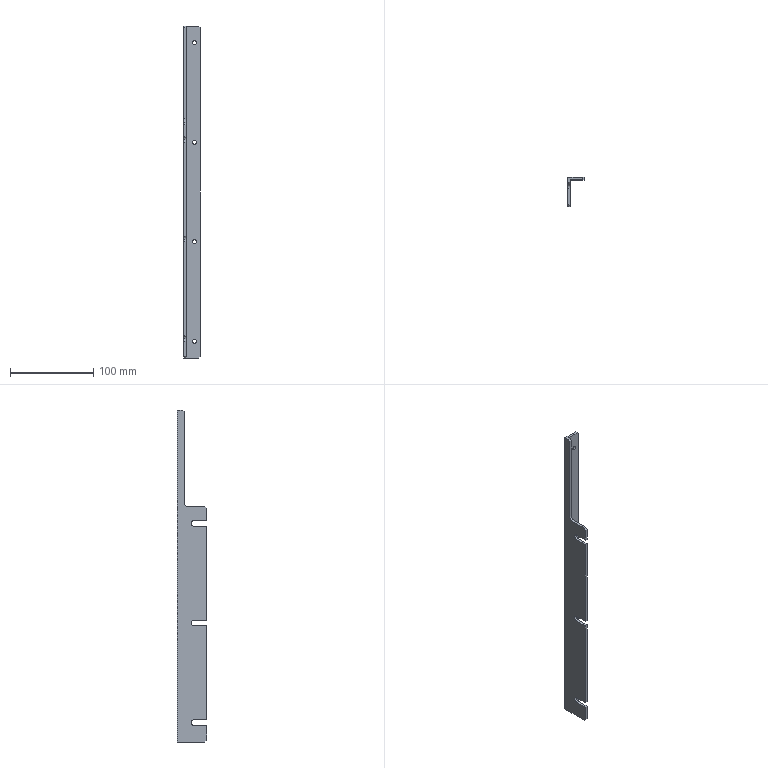Part | SolidWorks | features BaseBody 1 | 1 solid | 39 faces | box 20 x 35 x 400 mm | volume 51653 mm3 | plane 24 | cylinder 15 | commonest cylinder face diameters 5 x8 6.6 x6 10 x1
STEP:
#1=CARTESIAN_POINT('',(13.,32.,377.5));
#2=VERTEX_POINT('',#1);
#3=CARTESIAN_POINT('',(13.,32.,382.5));
#4=VERTEX_POINT('',#3);
#5=CARTESIAN_POINT('',(13.,32.,380.));
#6=DIRECTION('',(0.,1.,0.));
#7=DIRECTION('',(0.,0.,1.));
#8=AXIS2_PLACEMENT_3D('',#5,#6,#7);
#9=CIRCLE('',#8,2.5);
#10=EDGE_CURVE('',#2,#4,#9,.T.);
#11=ORIENTED_EDGE('',*,*,#10,.F.);
#12=CARTESIAN_POINT('',(13.,35.,377.5));
#13=VERTEX_POINT('',#12);
#14=CARTESIAN_POINT('',(13.,35.,377.5));
#15=DIRECTION('',(0.,1.,0.));
#16=VECTOR('',#15,1000.);
#17=LINE('',#14,#16);
#18=EDGE_CURVE('',#2,#13,#17,.T.);
#19=ORIENTED_EDGE('',*,*,#18,.T.);
#20=CARTESIAN_POINT('',(13.,35.,382.5));
#21=VERTEX_POINT('',#20);
#22=CARTESIAN_POINT('',(13.,35.,380.));
#23=DIRECTION('',(0.,1.,0.));
#24=DIRECTION('',(0.,0.,1.));
#25=AXIS2_PLACEMENT_3D('',#22,#23,#24);
#26=CIRCLE('',#25,2.5);
#27=EDGE_CURVE('',#13,#21,#26,.T.);
#28=ORIENTED_EDGE('',*,*,#27,.T.);
#29=CARTESIAN_POINT('',(13.,35.,382.5));
#30=DIRECTION('',(0.,1.,0.));
#31=VECTOR('',#30,1000.);
#32=LINE('',#29,#31);
#33=EDGE_CURVE('',#4,#21,#32,.T.);
#34=ORIENTED_EDGE('',*,*,#33,.F.);
#35=EDGE_LOOP('',(#11,#19,#28,#34));
#36=FACE_OUTER_BOUND('',#35,.T.);
#37=CARTESIAN_POINT('',(13.,35.,380.));
#38=DIRECTION('',(0.,1.,0.));
#39=DIRECTION('',(0.,0.,1.));
#40=AXIS2_PLACEMENT_3D('',#37,#38,#39);
#41=CYLINDRICAL_SURFACE('',#40,2.5);
#42=ADVANCED_FACE('',(#36),#41,.F.);
#43=CARTESIAN_POINT('',(13.,32.,257.5));
#44=VERTEX_POINT('',#43);
#45=CARTESIAN_POINT('',(13.,32.,262.5));
#46=VERTEX_POINT('',#45);
#47=CARTESIAN_POINT('',(13.,32.,260.));
#48=DIRECTION('',(0.,1.,0.));
#49=DIRECTION('',(0.,0.,1.));
#50=AXIS2_PLACEMENT_3D('',#47,#48,#49);
#51=CIRCLE('',#50,2.5);
#52=EDGE_CURVE('',#44,#46,#51,.T.);
#53=ORIENTED_EDGE('',*,*,#52,.F.);
#54=CARTESIAN_POINT('',(13.,35.,257.5));
#55=VERTEX_POINT('',#54);
#56=CARTESIAN_POINT('',(13.,35.,257.5));
#57=DIRECTION('',(0.,1.,0.));
#58=VECTOR('',#57,1000.);
#59=LINE('',#56,#58);
#60=EDGE_CURVE('',#44,#55,#59,.T.);
#61=ORIENTED_EDGE('',*,*,#60,.T.);
#62=CARTESIAN_POINT('',(13.,35.,262.5));
#63=VERTEX_POINT('',#62);
#64=CARTESIAN_POINT('',(13.,35.,260.));
#65=DIRECTION('',(0.,1.,0.));
#66=DIRECTION('',(0.,0.,1.));
#67=AXIS2_PLACEMENT_3D('',#64,#65,#66);
#68=CIRCLE('',#67,2.5);
#69=EDGE_CURVE('',#55,#63,#68,.T.);
#70=ORIENTED_EDGE('',*,*,#69,.T.);
#71=CARTESIAN_POINT('',(13.,35.,262.5));
#72=DIRECTION('',(0.,1.,0.));
#73=VECTOR('',#72,1000.);
#74=LINE('',#71,#73);
#75=EDGE_CURVE('',#46,#63,#74,.T.);
#76=ORIENTED_EDGE('',*,*,#75,.F.);
#77=EDGE_LOOP('',(#53,#61,#70,#76));
#78=FACE_OUTER_BOUND('',#77,.T.);
#79=CARTESIAN_POINT('',(13.,35.,260.));
#80=DIRECTION('',(0.,1.,0.));
#81=DIRECTION('',(0.,0.,1.));
#82=AXIS2_PLACEMENT_3D('',#79,#80,#81);
#83=CYLINDRICAL_SURFACE('',#82,2.5);
#84=ADVANCED_FACE('',(#78),#83,.F.);
#85=CARTESIAN_POINT('',(13.,32.,137.5));
#86=VERTEX_POINT('',#85);
#87=CARTESIAN_POINT('',(13.,32.,142.5));
#88=VERTEX_POINT('',#87);
#89=CARTESIAN_POINT('',(13.,32.,140.));
#90=DIRECTION('',(0.,1.,0.));
#91=DIRECTION('',(0.,0.,1.));
#92=AXIS2_PLACEMENT_3D('',#89,#90,#91);
#93=CIRCLE('',#92,2.5);
#94=EDGE_CURVE('',#86,#88,#93,.T.);
#95=ORIENTED_EDGE('',*,*,#94,.F.);
#96=CARTESIAN_POINT('',(13.,35.,137.5));
#97=VERTEX_POINT('',#96);
#98=CARTESIAN_POINT('',(13.,35.,137.5));
#99=DIRECTION('',(0.,1.,0.));
#100=VECTOR('',#99,1000.);
#101=LINE('',#98,#100);
#102=EDGE_CURVE('',#86,#97,#101,.T.);
#103=ORIENTED_EDGE('',*,*,#102,.T.);
#104=CARTESIAN_POINT('',(13.,35.,142.5));
#105=VERTEX_POINT('',#104);
#106=CARTESIAN_POINT('',(13.,35.,140.));
#107=DIRECTION('',(0.,1.,0.));
#108=DIRECTION('',(0.,0.,1.));
#109=AXIS2_PLACEMENT_3D('',#106,#107,#108);
#110=CIRCLE('',#109,2.5);
#111=EDGE_CURVE('',#97,#105,#110,.T.);
#112=ORIENTED_EDGE('',*,*,#111,.T.);
#113=CARTESIAN_POINT('',(13.,35.,142.5));
#114=DIRECTION('',(0.,1.,0.));
#115=VECTOR('',#114,1000.);
#116=LINE('',#113,#115);
#117=EDGE_CURVE('',#88,#105,#116,.T.);
#118=ORIENTED_EDGE('',*,*,#117,.F.);
#119=EDGE_LOOP('',(#95,#103,#112,#118));
#120=FACE_OUTER_BOUND('',#119,.T.);
#121=CARTESIAN_POINT('',(13.,35.,140.));
#122=DIRECTION('',(0.,1.,0.));
#123=DIRECTION('',(0.,0.,1.));
#124=AXIS2_PLACEMENT_3D('',#121,#122,#123);
#125=CYLINDRICAL_SURFACE('',#124,2.5);
#126=ADVANCED_FACE('',(#120),#125,.F.);
#127=CARTESIAN_POINT('',(13.,32.,17.5));
#128=VERTEX_POINT('',#127);
#129=CARTESIAN_POINT('',(13.,32.,22.5));
#130=VERTEX_POINT('',#129);
#131=CARTESIAN_POINT('',(13.,32.,20.));
#132=DIRECTION('',(0.,1.,0.));
#133=DIRECTION('',(0.,0.,1.));
#134=AXIS2_PLACEMENT_3D('',#131,#132,#133);
#135=CIRCLE('',#134,2.5);
#136=EDGE_CURVE('',#128,#130,#135,.T.);
#137=ORIENTED_EDGE('',*,*,#136,.F.);
#138=CARTESIAN_POINT('',(13.,35.,17.5));
#139=VERTEX_POINT('',#138);
#140=CARTESIAN_POINT('',(13.,35.,17.5));
#141=DIRECTION('',(0.,1.,0.));
#142=VECTOR('',#141,1000.);
#143=LINE('',#140,#142);
#144=EDGE_CURVE('',#128,#139,#143,.T.);
#145=ORIENTED_EDGE('',*,*,#144,.T.);
#146=CARTESIAN_POINT('',(13.,35.,22.5));
#147=VERTEX_POINT('',#146);
#148=CARTESIAN_POINT('',(13.,35.,20.));
#149=DIRECTION('',(0.,1.,0.));
#150=DIRECTION('',(0.,0.,1.));
#151=AXIS2_PLACEMENT_3D('',#148,#149,#150);
#152=CIRCLE('',#151,2.5);
#153=EDGE_CURVE('',#139,#147,#152,.T.);
#154=ORIENTED_EDGE('',*,*,#153,.T.);
#155=CARTESIAN_POINT('',(13.,35.,22.5));
#156=DIRECTION('',(0.,1.,0.));
#157=VECTOR('',#156,1000.);
#158=LINE('',#155,#157);
#159=EDGE_CURVE('',#130,#147,#158,.T.);
#160=ORIENTED_EDGE('',*,*,#159,.F.);
#161=EDGE_LOOP('',(#137,#145,#154,#160));
#162=FACE_OUTER_BOUND('',#161,.T.);
#163=CARTESIAN_POINT('',(13.,35.,20.));
#164=DIRECTION('',(0.,1.,0.));
#165=DIRECTION('',(0.,0.,1.));
#166=AXIS2_PLACEMENT_3D('',#163,#164,#165);
#167=CYLINDRICAL_SURFACE('',#166,2.5);
#168=ADVANCED_FACE('',(#162),#167,.F.);
#169=CARTESIAN_POINT('',(0.,18.3,23.3));
#170=VERTEX_POINT('',#169);
#171=CARTESIAN_POINT('',(0.,15.,26.6));
#172=VERTEX_POINT('',#171);
#173=CARTESIAN_POINT('',(0.,15.,23.3));
#174=DIRECTION('',(1.,0.,0.));
#175=DIRECTION('',(0.,1.,0.));
#176=AXIS2_PLACEMENT_3D('',#173,#174,#175);
#177=CIRCLE('',#176,3.3);
#178=EDGE_CURVE('',#170,#172,#177,.T.);
#179=ORIENTED_EDGE('',*,*,#178,.F.);
#180=CARTESIAN_POINT('',(3.,18.3,23.3));
#181=VERTEX_POINT('',#180);
#182=CARTESIAN_POINT('',(0.,18.3,23.3));
#183=DIRECTION('',(1.,0.,0.));
#184=VECTOR('',#183,1000.);
#185=LINE('',#182,#184);
#186=EDGE_CURVE('',#170,#181,#185,.T.);
#187=ORIENTED_EDGE('',*,*,#186,.T.);
#188=CARTESIAN_POINT('',(3.,15.,26.6));
#189=VERTEX_POINT('',#188);
#190=CARTESIAN_POINT('',(3.,15.,23.3));
#191=DIRECTION('',(1.,0.,0.));
#192=DIRECTION('',(0.,1.,0.));
#193=AXIS2_PLACEMENT_3D('',#190,#191,#192);
#194=CIRCLE('',#193,3.3);
#195=EDGE_CURVE('',#181,#189,#194,.T.);
#196=ORIENTED_EDGE('',*,*,#195,.T.);
#197=CARTESIAN_POINT('',(0.,15.,26.6));
#198=DIRECTION('',(1.,0.,0.));
#199=VECTOR('',#198,1000.);
#200=LINE('',#197,#199);
#201=EDGE_CURVE('',#172,#189,#200,.T.);
#202=ORIENTED_EDGE('',*,*,#201,.F.);
#203=EDGE_LOOP('',(#179,#187,#196,#202));
#204=FACE_OUTER_BOUND('',#203,.T.);
#205=CARTESIAN_POINT('',(0.,15.,23.3));
#206=DIRECTION('',(1.,0.,0.));
#207=DIRECTION('',(0.,1.,0.));
#208=AXIS2_PLACEMENT_3D('',#205,#206,#207);
#209=CYLINDRICAL_SURFACE('',#208,3.3);
#210=ADVANCED_FACE('',(#204),#209,.F.);
#211=CARTESIAN_POINT('',(0.,18.3,263.3));
#212=VERTEX_POINT('',#211);
#213=CARTESIAN_POINT('',(0.,15.,266.6));
#214=VERTEX_POINT('',#213);
#215=CARTESIAN_POINT('',(0.,15.,263.3));
#216=DIRECTION('',(1.,0.,0.));
#217=DIRECTION('',(0.,1.,0.));
#218=AXIS2_PLACEMENT_3D('',#215,#216,#217);
#219=CIRCLE('',#218,3.3);
#220=EDGE_CURVE('',#212,#214,#219,.T.);
#221=ORIENTED_EDGE('',*,*,#220,.F.);
#222=CARTESIAN_POINT('',(3.,18.3,263.3));
#223=VERTEX_POINT('',#222);
#224=CARTESIAN_POINT('',(0.,18.3,263.3));
#225=DIRECTION('',(1.,0.,0.));
#226=VECTOR('',#225,1000.);
#227=LINE('',#224,#226);
#228=EDGE_CURVE('',#212,#223,#227,.T.);
#229=ORIENTED_EDGE('',*,*,#228,.T.);
#230=CARTESIAN_POINT('',(3.,15.,266.6));
#231=VERTEX_POINT('',#230);
#232=CARTESIAN_POINT('',(3.,15.,263.3));
#233=DIRECTION('',(1.,0.,0.));
#234=DIRECTION('',(0.,1.,0.));
#235=AXIS2_PLACEMENT_3D('',#232,#233,#234);
#236=CIRCLE('',#235,3.3);
#237=EDGE_CURVE('',#223,#231,#236,.T.);
#238=ORIENTED_EDGE('',*,*,#237,.T.);
#239=CARTESIAN_POINT('',(0.,15.,266.6));
#240=DIRECTION('',(1.,0.,0.));
#241=VECTOR('',#240,1000.);
#242=LINE('',#239,#241);
#243=EDGE_CURVE('',#214,#231,#242,.T.);
#244=ORIENTED_EDGE('',*,*,#243,.F.);
#245=EDGE_LOOP('',(#221,#229,#238,#244));
#246=FACE_OUTER_BOUND('',#245,.T.);
#247=CARTESIAN_POINT('',(0.,15.,263.3));
#248=DIRECTION('',(1.,0.,0.));
#249=DIRECTION('',(0.,1.,0.));
#250=AXIS2_PLACEMENT_3D('',#247,#248,#249);
#251=CYLINDRICAL_SURFACE('',#250,3.3);
#252=ADVANCED_FACE('',(#246),#251,.F.);
#253=CARTESIAN_POINT('',(0.,18.3,143.3));
#254=VERTEX_POINT('',#253);
#255=CARTESIAN_POINT('',(0.,15.,146.6));
#256=VERTEX_POINT('',#255);
#257=CARTESIAN_POINT('',(0.,15.,143.3));
#258=DIRECTION('',(1.,0.,0.));
#259=DIRECTION('',(0.,1.,0.));
#260=AXIS2_PLACEMENT_3D('',#257,#258,#259);
#261=CIRCLE('',#260,3.3);
#262=EDGE_CURVE('',#254,#256,#261,.T.);
#263=ORIENTED_EDGE('',*,*,#262,.F.);
#264=CARTESIAN_POINT('',(3.,18.3,143.3));
#265=VERTEX_POINT('',#264);
#266=CARTESIAN_POINT('',(0.,18.3,143.3));
#267=DIRECTION('',(1.,0.,0.));
#268=VECTOR('',#267,1000.);
#269=LINE('',#266,#268);
#270=EDGE_CURVE('',#254,#265,#269,.T.);
#271=ORIENTED_EDGE('',*,*,#270,.T.);
#272=CARTESIAN_POINT('',(3.,15.,146.6));
#273=VERTEX_POINT('',#272);
#274=CARTESIAN_POINT('',(3.,15.,143.3));
#275=DIRECTION('',(1.,0.,0.));
#276=DIRECTION('',(0.,1.,0.));
#277=AXIS2_PLACEMENT_3D('',#274,#275,#276);
#278=CIRCLE('',#277,3.3);
#279=EDGE_CURVE('',#265,#273,#278,.T.);
#280=ORIENTED_EDGE('',*,*,#279,.T.);
#281=CARTESIAN_POINT('',(0.,15.,146.6));
#282=DIRECTION('',(1.,0.,0.));
#283=VECTOR('',#282,1000.);
#284=LINE('',#281,#283);
#285=EDGE_CURVE('',#256,#273,#284,.T.);
#286=ORIENTED_EDGE('',*,*,#285,.F.);
#287=EDGE_LOOP('',(#263,#271,#280,#286));
#288=FACE_OUTER_BOUND('',#287,.T.);
#289=CARTESIAN_POINT('',(0.,15.,143.3));
#290=DIRECTION('',(1.,0.,0.));
#291=DIRECTION('',(0.,1.,0.));
#292=AXIS2_PLACEMENT_3D('',#289,#290,#291);
#293=CYLINDRICAL_SURFACE('',#292,3.3);
#294=ADVANCED_FACE('',(#288),#293,.F.);
#295=CARTESIAN_POINT('',(0.,22.,283.3));
#296=VERTEX_POINT('',#295);
#297=CARTESIAN_POINT('',(0.,27.,288.3));
#298=VERTEX_POINT('',#297);
#299=CARTESIAN_POINT('',(0.,22.,288.3));
#300=DIRECTION('',(1.,0.,0.));
#301=DIRECTION('',(0.,0.,-1.));
#302=AXIS2_PLACEMENT_3D('',#299,#300,#301);
#303=CIRCLE('',#302,5.);
#304=EDGE_CURVE('',#296,#298,#303,.T.);
#305=ORIENTED_EDGE('',*,*,#304,.F.);
#306=CARTESIAN_POINT('',(3.,22.,283.3));
#307=VERTEX_POINT('',#306);
#308=CARTESIAN_POINT('',(0.,22.,283.3));
#309=DIRECTION('',(-1.,0.,0.));
#310=VECTOR('',#309,1000.);
#311=LINE('',#308,#310);
#312=EDGE_CURVE('',#307,#296,#311,.T.);
#313=ORIENTED_EDGE('',*,*,#312,.F.);
#314=CARTESIAN_POINT('',(3.,27.,288.3));
#315=VERTEX_POINT('',#314);
#316=CARTESIAN_POINT('',(3.,22.,288.3));
#317=DIRECTION('',(-1.,0.,0.));
#318=DIRECTION('',(0.,-1.,0.));
#319=AXIS2_PLACEMENT_3D('',#316,#317,#318);
#320=CIRCLE('',#319,5.);
#321=EDGE_CURVE('',#315,#307,#320,.T.);
#322=ORIENTED_EDGE('',*,*,#321,.F.);
#323=CARTESIAN_POINT('',(3.,27.,288.3));
#324=DIRECTION('',(1.,0.,0.));
#325=VECTOR('',#324,1000.);
#326=LINE('',#323,#325);
#327=EDGE_CURVE('',#298,#315,#326,.T.);
#328=ORIENTED_EDGE('',*,*,#327,.F.);
#329=EDGE_LOOP('',(#305,#313,#322,#328));
#330=FACE_OUTER_BOUND('',#329,.T.);
#331=CARTESIAN_POINT('',(0.,22.,288.3));
#332=DIRECTION('',(-1.,0.,0.));
#333=DIRECTION('',(0.,-1.,0.));
#334=AXIS2_PLACEMENT_3D('',#331,#332,#333);
#335=CYLINDRICAL_SURFACE('',#334,5.);
#336=ADVANCED_FACE('',(#330),#335,.F.);
#337=CARTESIAN_POINT('',(18.,32.,0.));
#338=VERTEX_POINT('',#337);
#339=CARTESIAN_POINT('',(20.,32.,2.));
#340=VERTEX_POINT('',#339);
#341=CARTESIAN_POINT('',(20.,32.,2.));
#342=DIRECTION('',(0.7071,0.,0.7071));
#343=VECTOR('',#342,1000.);
#344=LINE('',#341,#343);
#345=EDGE_CURVE('',#338,#340,#344,.T.);
#346=ORIENTED_EDGE('',*,*,#345,.F.);
#347=CARTESIAN_POINT('',(18.,35.,0.));
#348=VERTEX_POINT('',#347);
#349=CARTESIAN_POINT('',(18.,32.,0.));
#350=DIRECTION('',(0.,-1.,0.));
#351=VECTOR('',#350,1000.);
#352=LINE('',#349,#351);
#353=EDGE_CURVE('',#348,#338,#352,.T.);
#354=ORIENTED_EDGE('',*,*,#353,.F.);
#355=CARTESIAN_POINT('',(20.,35.,2.));
#356=VERTEX_POINT('',#355);
#357=CARTESIAN_POINT('',(20.,35.,2.));
#358=DIRECTION('',(-0.7071,0.,-0.7071));
#359=VECTOR('',#358,1000.);
#360=LINE('',#357,#359);
#361=EDGE_CURVE('',#356,#348,#360,.T.);
#362=ORIENTED_EDGE('',*,*,#361,.F.);
#363=CARTESIAN_POINT('',(20.,35.,2.));
#364=DIRECTION('',(0.,1.,0.));
#365=VECTOR('',#364,1000.);
#366=LINE('',#363,#365);
#367=EDGE_CURVE('',#340,#356,#366,.T.);
#368=ORIENTED_EDGE('',*,*,#367,.F.);
#369=EDGE_LOOP('',(#346,#354,#362,#368));
#370=FACE_OUTER_BOUND('',#369,.T.);
#371=CARTESIAN_POINT('',(20.,35.,2.));
#372=DIRECTION('',(0.7071,0.,-0.7071));
#373=DIRECTION('',(0.,-1.,0.));
#374=AXIS2_PLACEMENT_3D('',#371,#372,#373);
#375=PLANE('',#374);
#376=ADVANCED_FACE('',(#370),#375,.T.);
#377=CARTESIAN_POINT('',(20.,32.,398.));
#378=VERTEX_POINT('',#377);
#379=CARTESIAN_POINT('',(18.,32.,400.));
#380=VERTEX_POINT('',#379);
#381=CARTESIAN_POINT('',(18.,32.,400.));
#382=DIRECTION('',(-0.7071,0.,0.7071));
#383=VECTOR('',#382,1000.);
#384=LINE('',#381,#383);
#385=EDGE_CURVE('',#378,#380,#384,.T.);
#386=ORIENTED_EDGE('',*,*,#385,.F.);
#387=CARTESIAN_POINT('',(20.,35.,398.));
#388=VERTEX_POINT('',#387);
#389=CARTESIAN_POINT('',(20.,35.,398.));
#390=DIRECTION('',(0.,-1.,0.));
#391=VECTOR('',#390,1000.);
#392=LINE('',#389,#391);
#393=EDGE_CURVE('',#388,#378,#392,.T.);
#394=ORIENTED_EDGE('',*,*,#393,.F.);
#395=CARTESIAN_POINT('',(18.,35.,400.));
#396=VERTEX_POINT('',#395);
#397=CARTESIAN_POINT('',(18.,35.,400.));
#398=DIRECTION('',(0.7071,0.,-0.7071));
#399=VECTOR('',#398,1000.);
#400=LINE('',#397,#399);
#401=EDGE_CURVE('',#396,#388,#400,.T.);
#402=ORIENTED_EDGE('',*,*,#401,.F.);
#403=CARTESIAN_POINT('',(18.,0.,400.));
#404=DIRECTION('',(0.,1.,0.));
#405=VECTOR('',#404,1000.);
#406=LINE('',#403,#405);
#407=EDGE_CURVE('',#380,#396,#406,.T.);
#408=ORIENTED_EDGE('',*,*,#407,.F.);
#409=EDGE_LOOP('',(#386,#394,#402,#408));
#410=FACE_OUTER_BOUND('',#409,.T.);
#411=CARTESIAN_POINT('',(18.,0.,400.));
#412=DIRECTION('',(-0.7071,0.,-0.7071));
#413=DIRECTION('',(-0.7071,0.,0.7071));
#414=AXIS2_PLACEMENT_3D('',#411,#412,#413);
#415=PLANE('',#414);
#416=ADVANCED_FACE('',(#410),#415,.F.);
#417=CARTESIAN_POINT('',(0.,27.,398.));
#418=VERTEX_POINT('',#417);
#419=CARTESIAN_POINT('',(0.,29.,400.));
#420=VERTEX_POINT('',#419);
#421=CARTESIAN_POINT('',(0.,29.,400.));
#422=DIRECTION('',(0.,0.7071,0.7071));
#423=VECTOR('',#422,1000.);
#424=LINE('',#421,#423);
#425=EDGE_CURVE('',#418,#420,#424,.T.);
#426=ORIENTED_EDGE('',*,*,#425,.F.);
#427=CARTESIAN_POINT('',(3.,27.,398.));
#428=VERTEX_POINT('',#427);
#429=CARTESIAN_POINT('',(0.,27.,398.));
#430=DIRECTION('',(-1.,0.,0.));
#431=VECTOR('',#430,1000.);
#432=LINE('',#429,#431);
#433=EDGE_CURVE('',#428,#418,#432,.T.);
#434=ORIENTED_EDGE('',*,*,#433,.F.);
#435=CARTESIAN_POINT('',(3.,29.,400.));
#436=VERTEX_POINT('',#435);
#437=CARTESIAN_POINT('',(3.,29.,400.));
#438=DIRECTION('',(0.,-0.7071,-0.7071));
#439=VECTOR('',#438,1000.);
#440=LINE('',#437,#439);
#441=EDGE_CURVE('',#436,#428,#440,.T.);
#442=ORIENTED_EDGE('',*,*,#441,.F.);
#443=CARTESIAN_POINT('',(0.,29.,400.));
#444=DIRECTION('',(1.,0.,0.));
#445=VECTOR('',#444,1000.);
#446=LINE('',#443,#445);
#447=EDGE_CURVE('',#420,#436,#446,.T.);
#448=ORIENTED_EDGE('',*,*,#447,.F.);
#449=EDGE_LOOP('',(#426,#434,#442,#448));
#450=FACE_OUTER_BOUND('',#449,.T.);
#451=CARTESIAN_POINT('',(0.,29.,400.));
#452=DIRECTION('',(0.,0.7071,-0.7071));
#453=DIRECTION('',(-1.,0.,0.));
#454=AXIS2_PLACEMENT_3D('',#451,#452,#453);
#455=PLANE('',#454);
#456=ADVANCED_FACE('',(#450),#455,.F.);
#457=CARTESIAN_POINT('',(0.,0.,281.3));
#458=VERTEX_POINT('',#457);
#459=CARTESIAN_POINT('',(0.,2.,283.3));
#460=VERTEX_POINT('',#459);
#461=CARTESIAN_POINT('',(0.,2.,283.3));
#462=DIRECTION('',(0.,0.7071,0.7071));
#463=VECTOR('',#462,1000.);
#464=LINE('',#461,#463);
#465=EDGE_CURVE('',#458,#460,#464,.T.);
#466=ORIENTED_EDGE('',*,*,#465,.F.);
#467=CARTESIAN_POINT('',(3.,0.,281.3));
#468=VERTEX_POINT('',#467);
#469=CARTESIAN_POINT('',(3.,0.,281.3));
#470=DIRECTION('',(-1.,0.,0.));
#471=VECTOR('',#470,1000.);
#472=LINE('',#469,#471);
#473=EDGE_CURVE('',#468,#458,#472,.T.);
#474=ORIENTED_EDGE('',*,*,#473,.F.);
#475=CARTESIAN_POINT('',(3.,2.,283.3));
#476=VERTEX_POINT('',#475);
#477=CARTESIAN_POINT('',(3.,2.,283.3));
#478=DIRECTION('',(0.,-0.7071,-0.7071));
#479=VECTOR('',#478,1000.);
#480=LINE('',#477,#479);
#481=EDGE_CURVE('',#476,#468,#480,.T.);
#482=ORIENTED_EDGE('',*,*,#481,.F.);
#483=CARTESIAN_POINT('',(0.,2.,283.3));
#484=DIRECTION('',(1.,0.,0.));
#485=VECTOR('',#484,1000.);
#486=LINE('',#483,#485);
#487=EDGE_CURVE('',#460,#476,#486,.T.);
#488=ORIENTED_EDGE('',*,*,#487,.F.);
#489=EDGE_LOOP('',(#466,#474,#482,#488));
#490=FACE_OUTER_BOUND('',#489,.T.);
#491=CARTESIAN_POINT('',(0.,2.,283.3));
#492=DIRECTION('',(0.,0.7071,-0.7071));
#493=DIRECTION('',(-1.,0.,0.));
#494=AXIS2_PLACEMENT_3D('',#491,#492,#493);
#495=PLANE('',#494);
#496=ADVANCED_FACE('',(#490),#495,.F.);
#497=CARTESIAN_POINT('',(0.,2.,0.));
#498=VERTEX_POINT('',#497);
#499=CARTESIAN_POINT('',(0.,0.,2.));
#500=VERTEX_POINT('',#499);
#501=CARTESIAN_POINT('',(0.,0.,2.));
#502=DIRECTION('',(0.,-0.7071,0.7071));
#503=VECTOR('',#502,1000.);
#504=LINE('',#501,#503);
#505=EDGE_CURVE('',#498,#500,#504,.T.);
#506=ORIENTED_EDGE('',*,*,#505,.F.);
#507=CARTESIAN_POINT('',(3.,2.,0.));
#508=VERTEX_POINT('',#507);
#509=CARTESIAN_POINT('',(0.,2.,0.));
#510=DIRECTION('',(-1.,0.,0.));
#511=VECTOR('',#510,1000.);
#512=LINE('',#509,#511);
#513=EDGE_CURVE('',#508,#498,#512,.T.);
#514=ORIENTED_EDGE('',*,*,#513,.F.);
#515=CARTESIAN_POINT('',(3.,0.,2.));
#516=VERTEX_POINT('',#515);
#517=CARTESIAN_POINT('',(3.,0.,2.));
#518=DIRECTION('',(0.,0.7071,-0.7071));
#519=VECTOR('',#518,1000.);
#520=LINE('',#517,#519);
#521=EDGE_CURVE('',#516,#508,#520,.T.);
#522=ORIENTED_EDGE('',*,*,#521,.F.);
#523=CARTESIAN_POINT('',(3.,0.,2.));
#524=DIRECTION('',(1.,0.,0.));
#525=VECTOR('',#524,1000.);
#526=LINE('',#523,#525);
#527=EDGE_CURVE('',#500,#516,#526,.T.);
#528=ORIENTED_EDGE('',*,*,#527,.F.);
#529=EDGE_LOOP('',(#506,#514,#522,#528));
#530=FACE_OUTER_BOUND('',#529,.T.);
#531=CARTESIAN_POINT('',(3.,0.,2.));
#532=DIRECTION('',(0.,-0.7071,-0.7071));
#533=DIRECTION('',(0.,-0.7071,0.7071));
#534=AXIS2_PLACEMENT_3D('',#531,#532,#533);
#535=PLANE('',#534);
#536=ADVANCED_FACE('',(#530),#535,.T.);
#537=CARTESIAN_POINT('',(0.,27.,283.3));
#538=DIRECTION('',(0.,0.,1.));
#539=VECTOR('',#538,1000.);
#540=LINE('',#537,#539);
#541=EDGE_CURVE('',#298,#418,#540,.T.);
#542=ORIENTED_EDGE('',*,*,#541,.F.);
#543=ORIENTED_EDGE('',*,*,#327,.T.);
#544=CARTESIAN_POINT('',(3.,27.,283.3));
#545=DIRECTION('',(0.,0.,1.));
#546=VECTOR('',#545,1000.);
#547=LINE('',#544,#546);
#548=EDGE_CURVE('',#315,#428,#547,.T.);
#549=ORIENTED_EDGE('',*,*,#548,.T.);
#550=ORIENTED_EDGE('',*,*,#433,.T.);
#551=EDGE_LOOP('',(#542,#543,#549,#550));
#552=FACE_OUTER_BOUND('',#551,.T.);
#553=CARTESIAN_POINT('',(0.,27.,283.3));
#554=DIRECTION('',(0.,1.,0.));
#555=DIRECTION('',(0.,0.,-1.));
#556=AXIS2_PLACEMENT_3D('',#553,#554,#555);
#557=PLANE('',#556);
#558=ADVANCED_FACE('',(#552),#557,.F.);
#559=CARTESIAN_POINT('',(3.,0.,283.3));
#560=DIRECTION('',(0.,1.,0.));
#561=VECTOR('',#560,1000.);
#562=LINE('',#559,#561);
#563=EDGE_CURVE('',#476,#307,#562,.T.);
#564=ORIENTED_EDGE('',*,*,#563,.T.);
#565=ORIENTED_EDGE('',*,*,#312,.T.);
#566=CARTESIAN_POINT('',(0.,0.,283.3));
#567=DIRECTION('',(0.,1.,0.));
#568=VECTOR('',#567,1000.);
#569=LINE('',#566,#568);
#570=EDGE_CURVE('',#460,#296,#569,.T.);
#571=ORIENTED_EDGE('',*,*,#570,.F.);
#572=ORIENTED_EDGE('',*,*,#487,.T.);
#573=EDGE_LOOP('',(#564,#565,#571,#572));
#574=FACE_OUTER_BOUND('',#573,.T.);
#575=CARTESIAN_POINT('',(0.,0.,283.3));
#576=DIRECTION('',(0.,0.,-1.));
#577=DIRECTION('',(0.,-1.,0.));
#578=AXIS2_PLACEMENT_3D('',#575,#576,#577);
#579=PLANE('',#578);
#580=ADVANCED_FACE('',(#574),#579,.F.);
#581=CARTESIAN_POINT('',(3.,0.,20.));
#582=VERTEX_POINT('',#581);
#583=CARTESIAN_POINT('',(3.,15.,20.));
#584=VERTEX_POINT('',#583);
#585=CARTESIAN_POINT('',(3.,0.,20.));
#586=DIRECTION('',(0.,1.,0.));
#587=VECTOR('',#586,1000.);
#588=LINE('',#585,#587);
#589=EDGE_CURVE('',#582,#584,#588,.T.);
#590=ORIENTED_EDGE('',*,*,#589,.T.);
#591=CARTESIAN_POINT('',(0.,15.,20.));
#592=VERTEX_POINT('',#591);
#593=CARTESIAN_POINT('',(0.,15.,20.));
#594=DIRECTION('',(1.,0.,0.));
#595=VECTOR('',#594,1000.);
#596=LINE('',#593,#595);
#597=EDGE_CURVE('',#592,#584,#596,.T.);
#598=ORIENTED_EDGE('',*,*,#597,.F.);
#599=CARTESIAN_POINT('',(0.,0.,20.));
#600=VERTEX_POINT('',#599);
#601=CARTESIAN_POINT('',(0.,0.,20.));
#602=DIRECTION('',(0.,1.,0.));
#603=VECTOR('',#602,1000.);
#604=LINE('',#601,#603);
#605=EDGE_CURVE('',#600,#592,#604,.T.);
#606=ORIENTED_EDGE('',*,*,#605,.F.);
#607=CARTESIAN_POINT('',(0.,0.,20.));
#608=DIRECTION('',(1.,0.,0.));
#609=VECTOR('',#608,1000.);
#610=LINE('',#607,#609);
#611=EDGE_CURVE('',#600,#582,#610,.T.);
#612=ORIENTED_EDGE('',*,*,#611,.T.);
#613=EDGE_LOOP('',(#590,#598,#606,#612));
#614=FACE_OUTER_BOUND('',#613,.T.);
#615=CARTESIAN_POINT('',(0.,0.,20.));
#616=DIRECTION('',(0.,0.,-1.));
#617=DIRECTION('',(0.,-1.,0.));
#618=AXIS2_PLACEMENT_3D('',#615,#616,#617);
#619=PLANE('',#618);
#620=ADVANCED_FACE('',(#614),#619,.F.);
#621=CARTESIAN_POINT('',(3.,0.,26.6));
#622=VERTEX_POINT('',#621);
#623=CARTESIAN_POINT('',(3.,0.,26.6));
#624=DIRECTION('',(0.,-1.,0.));
#625=VECTOR('',#624,1000.);
#626=LINE('',#623,#625);
#627=EDGE_CURVE('',#189,#622,#626,.T.);
#628=ORIENTED_EDGE('',*,*,#627,.T.);
#629=CARTESIAN_POINT('',(0.,0.,26.6));
#630=VERTEX_POINT('',#629);
#631=CARTESIAN_POINT('',(0.,0.,26.6));
#632=DIRECTION('',(1.,0.,0.));
#633=VECTOR('',#632,1000.);
#634=LINE('',#631,#633);
#635=EDGE_CURVE('',#630,#622,#634,.T.);
#636=ORIENTED_EDGE('',*,*,#635,.F.);
#637=CARTESIAN_POINT('',(0.,0.,26.6));
#638=DIRECTION('',(0.,-1.,0.));
#639=VECTOR('',#638,1000.);
#640=LINE('',#637,#639);
#641=EDGE_CURVE('',#172,#630,#640,.T.);
#642=ORIENTED_EDGE('',*,*,#641,.F.);
#643=ORIENTED_EDGE('',*,*,#201,.T.);
#644=EDGE_LOOP('',(#628,#636,#642,#643));
#645=FACE_OUTER_BOUND('',#644,.T.);
#646=CARTESIAN_POINT('',(0.,0.,26.6));
#647=DIRECTION('',(0.,0.,1.));
#648=DIRECTION('',(0.,-1.,0.));
#649=AXIS2_PLACEMENT_3D('',#646,#647,#648);
#650=PLANE('',#649);
#651=ADVANCED_FACE('',(#645),#650,.F.);
#652=CARTESIAN_POINT('',(3.,0.,260.));
#653=VERTEX_POINT('',#652);
#654=CARTESIAN_POINT('',(3.,15.,260.));
#655=VERTEX_POINT('',#654);
#656=CARTESIAN_POINT('',(3.,0.,260.));
#657=DIRECTION('',(0.,1.,0.));
#658=VECTOR('',#657,1000.);
#659=LINE('',#656,#658);
#660=EDGE_CURVE('',#653,#655,#659,.T.);
#661=ORIENTED_EDGE('',*,*,#660,.T.);
#662=CARTESIAN_POINT('',(0.,15.,260.));
#663=VERTEX_POINT('',#662);
#664=CARTESIAN_POINT('',(0.,15.,260.));
#665=DIRECTION('',(1.,0.,0.));
#666=VECTOR('',#665,1000.);
#667=LINE('',#664,#666);
#668=EDGE_CURVE('',#663,#655,#667,.T.);
#669=ORIENTED_EDGE('',*,*,#668,.F.);
#670=CARTESIAN_POINT('',(0.,0.,260.));
#671=VERTEX_POINT('',#670);
#672=CARTESIAN_POINT('',(0.,0.,260.));
#673=DIRECTION('',(0.,1.,0.));
#674=VECTOR('',#673,1000.);
#675=LINE('',#672,#674);
#676=EDGE_CURVE('',#671,#663,#675,.T.);
#677=ORIENTED_EDGE('',*,*,#676,.F.);
#678=CARTESIAN_POINT('',(0.,0.,260.));
#679=DIRECTION('',(1.,0.,0.));
#680=VECTOR('',#679,1000.);
#681=LINE('',#678,#680);
#682=EDGE_CURVE('',#671,#653,#681,.T.);
#683=ORIENTED_EDGE('',*,*,#682,.T.);
#684=EDGE_LOOP('',(#661,#669,#677,#683));
#685=FACE_OUTER_BOUND('',#684,.T.);
#686=CARTESIAN_POINT('',(0.,0.,260.));
#687=DIRECTION('',(0.,0.,-1.));
#688=DIRECTION('',(0.,-1.,0.));
#689=AXIS2_PLACEMENT_3D('',#686,#687,#688);
#690=PLANE('',#689);
#691=ADVANCED_FACE('',(#685),#690,.F.);
#692=CARTESIAN_POINT('',(3.,0.,266.6));
#693=VERTEX_POINT('',#692);
#694=CARTESIAN_POINT('',(3.,0.,266.6));
#695=DIRECTION('',(0.,-1.,0.));
#696=VECTOR('',#695,1000.);
#697=LINE('',#694,#696);
#698=EDGE_CURVE('',#231,#693,#697,.T.);
#699=ORIENTED_EDGE('',*,*,#698,.T.);
#700=CARTESIAN_POINT('',(0.,0.,266.6));
#701=VERTEX_POINT('',#700);
#702=CARTESIAN_POINT('',(0.,0.,266.6));
#703=DIRECTION('',(1.,0.,0.));
#704=VECTOR('',#703,1000.);
#705=LINE('',#702,#704);
#706=EDGE_CURVE('',#701,#693,#705,.T.);
#707=ORIENTED_EDGE('',*,*,#706,.F.);
#708=CARTESIAN_POINT('',(0.,0.,266.6));
#709=DIRECTION('',(0.,-1.,0.));
#710=VECTOR('',#709,1000.);
#711=LINE('',#708,#710);
#712=EDGE_CURVE('',#214,#701,#711,.T.);
#713=ORIENTED_EDGE('',*,*,#712,.F.);
#714=ORIENTED_EDGE('',*,*,#243,.T.);
#715=EDGE_LOOP('',(#699,#707,#713,#714));
#716=FACE_OUTER_BOUND('',#715,.T.);
#717=CARTESIAN_POINT('',(0.,0.,266.6));
#718=DIRECTION('',(0.,0.,1.));
#719=DIRECTION('',(1.,0.,0.));
#720=AXIS2_PLACEMENT_3D('',#717,#718,#719);
#721=PLANE('',#720);
#722=ADVANCED_FACE('',(#716),#721,.F.);
#723=CARTESIAN_POINT('',(3.,0.,146.6));
#724=VERTEX_POINT('',#723);
#725=CARTESIAN_POINT('',(3.,15.,146.6));
#726=DIRECTION('',(0.,-1.,0.));
#727=VECTOR('',#726,1000.);
#728=LINE('',#725,#727);
#729=EDGE_CURVE('',#273,#724,#728,.T.);
#730=ORIENTED_EDGE('',*,*,#729,.T.);
#731=CARTESIAN_POINT('',(0.,0.,146.6));
#732=VERTEX_POINT('',#731);
#733=CARTESIAN_POINT('',(0.,0.,146.6));
#734=DIRECTION('',(1.,0.,0.));
#735=VECTOR('',#734,1000.);
#736=LINE('',#733,#735);
#737=EDGE_CURVE('',#732,#724,#736,.T.);
#738=ORIENTED_EDGE('',*,*,#737,.F.);
#739=CARTESIAN_POINT('',(0.,15.,146.6));
#740=DIRECTION('',(0.,-1.,0.));
#741=VECTOR('',#740,1000.);
#742=LINE('',#739,#741);
#743=EDGE_CURVE('',#256,#732,#742,.T.);
#744=ORIENTED_EDGE('',*,*,#743,.F.);
#745=ORIENTED_EDGE('',*,*,#285,.T.);
#746=EDGE_LOOP('',(#730,#738,#744,#745));
#747=FACE_OUTER_BOUND('',#746,.T.);
#748=CARTESIAN_POINT('',(0.,15.,146.6));
#749=DIRECTION('',(0.,0.,1.));
#750=DIRECTION('',(1.,0.,0.));
#751=AXIS2_PLACEMENT_3D('',#748,#749,#750);
#752=PLANE('',#751);
#753=ADVANCED_FACE('',(#747),#752,.F.);
#754=CARTESIAN_POINT('',(3.,0.,140.));
#755=VERTEX_POINT('',#754);
#756=CARTESIAN_POINT('',(3.,15.,140.));
#757=VERTEX_POINT('',#756);
#758=CARTESIAN_POINT('',(3.,15.,140.));
#759=DIRECTION('',(0.,1.,0.));
#760=VECTOR('',#759,1000.);
#761=LINE('',#758,#760);
#762=EDGE_CURVE('',#755,#757,#761,.T.);
#763=ORIENTED_EDGE('',*,*,#762,.T.);
#764=CARTESIAN_POINT('',(0.,15.,140.));
#765=VERTEX_POINT('',#764);
#766=CARTESIAN_POINT('',(0.,15.,140.));
#767=DIRECTION('',(1.,0.,0.));
#768=VECTOR('',#767,1000.);
#769=LINE('',#766,#768);
#770=EDGE_CURVE('',#765,#757,#769,.T.);
#771=ORIENTED_EDGE('',*,*,#770,.F.);
#772=CARTESIAN_POINT('',(0.,0.,140.));
#773=VERTEX_POINT('',#772);
#774=CARTESIAN_POINT('',(0.,15.,140.));
#775=DIRECTION('',(0.,1.,0.));
#776=VECTOR('',#775,1000.);
#777=LINE('',#774,#776);
#778=EDGE_CURVE('',#773,#765,#777,.T.);
#779=ORIENTED_EDGE('',*,*,#778,.F.);
#780=CARTESIAN_POINT('',(0.,0.,140.));
#781=DIRECTION('',(1.,0.,0.));
#782=VECTOR('',#781,1000.);
#783=LINE('',#780,#782);
#784=EDGE_CURVE('',#773,#755,#783,.T.);
#785=ORIENTED_EDGE('',*,*,#784,.T.);
#786=EDGE_LOOP('',(#763,#771,#779,#785));
#787=FACE_OUTER_BOUND('',#786,.T.);
#788=CARTESIAN_POINT('',(0.,15.,140.));
#789=DIRECTION('',(0.,0.,-1.));
#790=DIRECTION('',(0.,-1.,0.));
#791=AXIS2_PLACEMENT_3D('',#788,#789,#790);
#792=PLANE('',#791);
#793=ADVANCED_FACE('',(#787),#792,.F.);
#794=CARTESIAN_POINT('',(3.,32.,0.));
#795=VERTEX_POINT('',#794);
#796=CARTESIAN_POINT('',(3.,32.,0.));
#797=DIRECTION('',(0.,1.,0.));
#798=VECTOR('',#797,1000.);
#799=LINE('',#796,#798);
#800=EDGE_CURVE('',#508,#795,#799,.T.);
#801=ORIENTED_EDGE('',*,*,#800,.F.);
#802=ORIENTED_EDGE('',*,*,#513,.T.);
#803=CARTESIAN_POINT('',(0.,35.,0.));
#804=VERTEX_POINT('',#803);
#805=CARTESIAN_POINT('',(0.,0.,0.));
#806=DIRECTION('',(0.,-1.,0.));
#807=VECTOR('',#806,1000.);
#808=LINE('',#805,#807);
#809=EDGE_CURVE('',#804,#498,#808,.T.);
#810=ORIENTED_EDGE('',*,*,#809,.F.);
#811=CARTESIAN_POINT('',(0.,35.,0.));
#812=DIRECTION('',(-1.,0.,0.));
#813=VECTOR('',#812,1000.);
#814=LINE('',#811,#813);
#815=EDGE_CURVE('',#348,#804,#814,.T.);
#816=ORIENTED_EDGE('',*,*,#815,.F.);
#817=ORIENTED_EDGE('',*,*,#353,.T.);
#818=CARTESIAN_POINT('',(20.,32.,0.));
#819=DIRECTION('',(1.,0.,0.));
#820=VECTOR('',#819,1000.);
#821=LINE('',#818,#820);
#822=EDGE_CURVE('',#795,#338,#821,.T.);
#823=ORIENTED_EDGE('',*,*,#822,.F.);
#824=EDGE_LOOP('',(#801,#802,#810,#816,#817,#823));
#825=FACE_OUTER_BOUND('',#824,.T.);
#826=CARTESIAN_POINT('',(0.,0.,0.));
#827=DIRECTION('',(0.,0.,-1.));
#828=DIRECTION('',(0.,-1.,0.));
#829=AXIS2_PLACEMENT_3D('',#826,#827,#828);
#830=PLANE('',#829);
#831=ADVANCED_FACE('',(#825),#830,.T.);
#832=CARTESIAN_POINT('',(0.,35.,400.));
#833=VERTEX_POINT('',#832);
#834=CARTESIAN_POINT('',(0.,0.,400.));
#835=DIRECTION('',(0.,-1.,0.));
#836=VECTOR('',#835,1000.);
#837=LINE('',#834,#836);
#838=EDGE_CURVE('',#833,#420,#837,.T.);
#839=ORIENTED_EDGE('',*,*,#838,.T.);
#840=ORIENTED_EDGE('',*,*,#447,.T.);
#841=CARTESIAN_POINT('',(3.,32.,400.));
#842=VERTEX_POINT('',#841);
#843=CARTESIAN_POINT('',(3.,32.,400.));
#844=DIRECTION('',(0.,1.,0.));
#845=VECTOR('',#844,1000.);
#846=LINE('',#843,#845);
#847=EDGE_CURVE('',#436,#842,#846,.T.);
#848=ORIENTED_EDGE('',*,*,#847,.T.);
#849=CARTESIAN_POINT('',(20.,32.,400.));
#850=DIRECTION('',(1.,0.,0.));
#851=VECTOR('',#850,1000.);
#852=LINE('',#849,#851);
#853=EDGE_CURVE('',#842,#380,#852,.T.);
#854=ORIENTED_EDGE('',*,*,#853,.T.);
#855=ORIENTED_EDGE('',*,*,#407,.T.);
#856=CARTESIAN_POINT('',(0.,35.,400.));
#857=DIRECTION('',(-1.,0.,0.));
#858=VECTOR('',#857,1000.);
#859=LINE('',#856,#858);
#860=EDGE_CURVE('',#396,#833,#859,.T.);
#861=ORIENTED_EDGE('',*,*,#860,.T.);
#862=EDGE_LOOP('',(#839,#840,#848,#854,#855,#861));
#863=FACE_OUTER_BOUND('',#862,.T.);
#864=CARTESIAN_POINT('',(0.,0.,400.));
#865=DIRECTION('',(0.,0.,-1.));
#866=DIRECTION('',(0.,-1.,0.));
#867=AXIS2_PLACEMENT_3D('',#864,#865,#866);
#868=PLANE('',#867);
#869=ADVANCED_FACE('',(#863),#868,.F.);
#870=ORIENTED_EDGE('',*,*,#809,.T.);
#871=ORIENTED_EDGE('',*,*,#505,.T.);
#872=CARTESIAN_POINT('',(0.,0.,400.));
#873=DIRECTION('',(0.,0.,-1.));
#874=VECTOR('',#873,1000.);
#875=LINE('',#872,#874);
#876=EDGE_CURVE('',#600,#500,#875,.T.);
#877=ORIENTED_EDGE('',*,*,#876,.F.);
#878=ORIENTED_EDGE('',*,*,#605,.T.);
#879=CARTESIAN_POINT('',(0.,15.,23.3));
#880=DIRECTION('',(1.,0.,0.));
#881=DIRECTION('',(0.,1.,0.));
#882=AXIS2_PLACEMENT_3D('',#879,#880,#881);
#883=CIRCLE('',#882,3.3);
#884=EDGE_CURVE('',#592,#170,#883,.T.);
#885=ORIENTED_EDGE('',*,*,#884,.T.);
#886=ORIENTED_EDGE('',*,*,#178,.T.);
#887=ORIENTED_EDGE('',*,*,#641,.T.);
#888=CARTESIAN_POINT('',(0.,0.,400.));
#889=DIRECTION('',(0.,0.,-1.));
#890=VECTOR('',#889,1000.);
#891=LINE('',#888,#890);
#892=EDGE_CURVE('',#773,#630,#891,.T.);
#893=ORIENTED_EDGE('',*,*,#892,.F.);
#894=ORIENTED_EDGE('',*,*,#778,.T.);
#895=CARTESIAN_POINT('',(0.,15.,143.3));
#896=DIRECTION('',(1.,0.,0.));
#897=DIRECTION('',(0.,1.,0.));
#898=AXIS2_PLACEMENT_3D('',#895,#896,#897);
#899=CIRCLE('',#898,3.3);
#900=EDGE_CURVE('',#765,#254,#899,.T.);
#901=ORIENTED_EDGE('',*,*,#900,.T.);
#902=ORIENTED_EDGE('',*,*,#262,.T.);
#903=ORIENTED_EDGE('',*,*,#743,.T.);
#904=CARTESIAN_POINT('',(0.,0.,400.));
#905=DIRECTION('',(0.,0.,-1.));
#906=VECTOR('',#905,1000.);
#907=LINE('',#904,#906);
#908=EDGE_CURVE('',#671,#732,#907,.T.);
#909=ORIENTED_EDGE('',*,*,#908,.F.);
#910=ORIENTED_EDGE('',*,*,#676,.T.);
#911=CARTESIAN_POINT('',(0.,15.,263.3));
#912=DIRECTION('',(1.,0.,0.));
#913=DIRECTION('',(0.,1.,0.));
#914=AXIS2_PLACEMENT_3D('',#911,#912,#913);
#915=CIRCLE('',#914,3.3);
#916=EDGE_CURVE('',#663,#212,#915,.T.);
#917=ORIENTED_EDGE('',*,*,#916,.T.);
#918=ORIENTED_EDGE('',*,*,#220,.T.);
#919=ORIENTED_EDGE('',*,*,#712,.T.);
#920=CARTESIAN_POINT('',(0.,0.,400.));
#921=DIRECTION('',(0.,0.,-1.));
#922=VECTOR('',#921,1000.);
#923=LINE('',#920,#922);
#924=EDGE_CURVE('',#458,#701,#923,.T.);
#925=ORIENTED_EDGE('',*,*,#924,.F.);
#926=ORIENTED_EDGE('',*,*,#465,.T.);
#927=ORIENTED_EDGE('',*,*,#570,.T.);
#928=ORIENTED_EDGE('',*,*,#304,.T.);
#929=ORIENTED_EDGE('',*,*,#541,.T.);
#930=ORIENTED_EDGE('',*,*,#425,.T.);
#931=ORIENTED_EDGE('',*,*,#838,.F.);
#932=CARTESIAN_POINT('',(0.,35.,400.));
#933=DIRECTION('',(0.,0.,-1.));
#934=VECTOR('',#933,1000.);
#935=LINE('',#932,#934);
#936=EDGE_CURVE('',#833,#804,#935,.T.);
#937=ORIENTED_EDGE('',*,*,#936,.T.);
#938=EDGE_LOOP('',(#870,#871,#877,#878,#885,#886,#887,#893,#894,#901,#902,#903,#909,#910,#917,#918,#919,#925,#926,#927,#928,#929,#930,#931,#937));
#939=FACE_OUTER_BOUND('',#938,.T.);
#940=CARTESIAN_POINT('',(0.,0.,400.));
#941=DIRECTION('',(1.,0.,0.));
#942=DIRECTION('',(0.,1.,0.));
#943=AXIS2_PLACEMENT_3D('',#940,#941,#942);
#944=PLANE('',#943);
#945=ADVANCED_FACE('',(#939),#944,.F.);
#946=CARTESIAN_POINT('',(13.,35.,20.));
#947=DIRECTION('',(0.,1.,0.));
#948=DIRECTION('',(0.,0.,1.));
#949=AXIS2_PLACEMENT_3D('',#946,#947,#948);
#950=CIRCLE('',#949,2.5);
#951=EDGE_CURVE('',#147,#139,#950,.T.);
#952=ORIENTED_EDGE('',*,*,#951,.F.);
#953=ORIENTED_EDGE('',*,*,#153,.F.);
#954=EDGE_LOOP('',(#952,#953));
#955=FACE_BOUND('',#954,.T.);
#956=CARTESIAN_POINT('',(13.,35.,140.));
#957=DIRECTION('',(0.,1.,0.));
#958=DIRECTION('',(0.,0.,1.));
#959=AXIS2_PLACEMENT_3D('',#956,#957,#958);
#960=CIRCLE('',#959,2.5);
#961=EDGE_CURVE('',#105,#97,#960,.T.);
#962=ORIENTED_EDGE('',*,*,#961,.F.);
#963=ORIENTED_EDGE('',*,*,#111,.F.);
#964=EDGE_LOOP('',(#962,#963));
#965=FACE_BOUND('',#964,.T.);
#966=CARTESIAN_POINT('',(13.,35.,260.));
#967=DIRECTION('',(0.,1.,0.));
#968=DIRECTION('',(0.,0.,1.));
#969=AXIS2_PLACEMENT_3D('',#966,#967,#968);
#970=CIRCLE('',#969,2.5);
#971=EDGE_CURVE('',#63,#55,#970,.T.);
#972=ORIENTED_EDGE('',*,*,#971,.F.);
#973=ORIENTED_EDGE('',*,*,#69,.F.);
#974=EDGE_LOOP('',(#972,#973));
#975=FACE_BOUND('',#974,.T.);
#976=CARTESIAN_POINT('',(13.,35.,380.));
#977=DIRECTION('',(0.,1.,0.));
#978=DIRECTION('',(0.,0.,1.));
#979=AXIS2_PLACEMENT_3D('',#976,#977,#978);
#980=CIRCLE('',#979,2.5);
#981=EDGE_CURVE('',#21,#13,#980,.T.);
#982=ORIENTED_EDGE('',*,*,#981,.F.);
#983=ORIENTED_EDGE('',*,*,#27,.F.);
#984=EDGE_LOOP('',(#982,#983));
#985=FACE_BOUND('',#984,.T.);
#986=ORIENTED_EDGE('',*,*,#860,.F.);
#987=ORIENTED_EDGE('',*,*,#401,.T.);
#988=CARTESIAN_POINT('',(20.,35.,400.));
#989=DIRECTION('',(0.,0.,-1.));
#990=VECTOR('',#989,1000.);
#991=LINE('',#988,#990);
#992=EDGE_CURVE('',#388,#356,#991,.T.);
#993=ORIENTED_EDGE('',*,*,#992,.T.);
#994=ORIENTED_EDGE('',*,*,#361,.T.);
#995=ORIENTED_EDGE('',*,*,#815,.T.);
#996=ORIENTED_EDGE('',*,*,#936,.F.);
#997=EDGE_LOOP('',(#986,#987,#993,#994,#995,#996));
#998=FACE_OUTER_BOUND('',#997,.T.);
#999=CARTESIAN_POINT('',(0.,35.,400.));
#1000=DIRECTION('',(0.,-1.,0.));
#1001=DIRECTION('',(0.,0.,-1.));
#1002=AXIS2_PLACEMENT_3D('',#999,#1000,#1001);
#1003=PLANE('',#1002);
#1004=ADVANCED_FACE('',(#955,#965,#975,#985,#998),#1003,.F.);
#1005=ORIENTED_EDGE('',*,*,#992,.F.);
#1006=ORIENTED_EDGE('',*,*,#393,.T.);
#1007=CARTESIAN_POINT('',(20.,32.,400.));
#1008=DIRECTION('',(0.,0.,-1.));
#1009=VECTOR('',#1008,1000.);
#1010=LINE('',#1007,#1009);
#1011=EDGE_CURVE('',#378,#340,#1010,.T.);
#1012=ORIENTED_EDGE('',*,*,#1011,.T.);
#1013=ORIENTED_EDGE('',*,*,#367,.T.);
#1014=EDGE_LOOP('',(#1005,#1006,#1012,#1013));
#1015=FACE_OUTER_BOUND('',#1014,.T.);
#1016=CARTESIAN_POINT('',(20.,35.,400.));
#1017=DIRECTION('',(-1.,0.,0.));
#1018=DIRECTION('',(0.,0.,1.));
#1019=AXIS2_PLACEMENT_3D('',#1016,#1017,#1018);
#1020=PLANE('',#1019);
#1021=ADVANCED_FACE('',(#1015),#1020,.F.);
#1022=CARTESIAN_POINT('',(13.,32.,20.));
#1023=DIRECTION('',(0.,1.,0.));
#1024=DIRECTION('',(0.,0.,1.));
#1025=AXIS2_PLACEMENT_3D('',#1022,#1023,#1024);
#1026=CIRCLE('',#1025,2.5);
#1027=EDGE_CURVE('',#130,#128,#1026,.T.);
#1028=ORIENTED_EDGE('',*,*,#1027,.T.);
#1029=ORIENTED_EDGE('',*,*,#136,.T.);
#1030=EDGE_LOOP('',(#1028,#1029));
#1031=FACE_BOUND('',#1030,.T.);
#1032=CARTESIAN_POINT('',(13.,32.,140.));
#1033=DIRECTION('',(0.,1.,0.));
#1034=DIRECTION('',(0.,0.,1.));
#1035=AXIS2_PLACEMENT_3D('',#1032,#1033,#1034);
#1036=CIRCLE('',#1035,2.5);
#1037=EDGE_CURVE('',#88,#86,#1036,.T.);
#1038=ORIENTED_EDGE('',*,*,#1037,.T.);
#1039=ORIENTED_EDGE('',*,*,#94,.T.);
#1040=EDGE_LOOP('',(#1038,#1039));
#1041=FACE_BOUND('',#1040,.T.);
#1042=CARTESIAN_POINT('',(13.,32.,260.));
#1043=DIRECTION('',(0.,1.,0.));
#1044=DIRECTION('',(0.,0.,1.));
#1045=AXIS2_PLACEMENT_3D('',#1042,#1043,#1044);
#1046=CIRCLE('',#1045,2.5);
#1047=EDGE_CURVE('',#46,#44,#1046,.T.);
#1048=ORIENTED_EDGE('',*,*,#1047,.T.);
#1049=ORIENTED_EDGE('',*,*,#52,.T.);
#1050=EDGE_LOOP('',(#1048,#1049));
#1051=FACE_BOUND('',#1050,.T.);
#1052=CARTESIAN_POINT('',(13.,32.,380.));
#1053=DIRECTION('',(0.,1.,0.));
#1054=DIRECTION('',(0.,0.,1.));
#1055=AXIS2_PLACEMENT_3D('',#1052,#1053,#1054);
#1056=CIRCLE('',#1055,2.5);
#1057=EDGE_CURVE('',#4,#2,#1056,.T.);
#1058=ORIENTED_EDGE('',*,*,#1057,.T.);
#1059=ORIENTED_EDGE('',*,*,#10,.T.);
#1060=EDGE_LOOP('',(#1058,#1059));
#1061=FACE_BOUND('',#1060,.T.);
#1062=ORIENTED_EDGE('',*,*,#1011,.F.);
#1063=ORIENTED_EDGE('',*,*,#385,.T.);
#1064=ORIENTED_EDGE('',*,*,#853,.F.);
#1065=CARTESIAN_POINT('',(3.,32.,400.));
#1066=DIRECTION('',(0.,0.,-1.));
#1067=VECTOR('',#1066,1000.);
#1068=LINE('',#1065,#1067);
#1069=EDGE_CURVE('',#842,#795,#1068,.T.);
#1070=ORIENTED_EDGE('',*,*,#1069,.T.);
#1071=ORIENTED_EDGE('',*,*,#822,.T.);
#1072=ORIENTED_EDGE('',*,*,#345,.T.);
#1073=EDGE_LOOP('',(#1062,#1063,#1064,#1070,#1071,#1072));
#1074=FACE_OUTER_BOUND('',#1073,.T.);
#1075=CARTESIAN_POINT('',(20.,32.,400.));
#1076=DIRECTION('',(0.,1.,0.));
#1077=DIRECTION('',(1.,0.,0.));
#1078=AXIS2_PLACEMENT_3D('',#1075,#1076,#1077);
#1079=PLANE('',#1078);
#1080=ADVANCED_FACE('',(#1031,#1041,#1051,#1061,#1074),#1079,.F.);
#1081=CARTESIAN_POINT('',(3.,0.,400.));
#1082=DIRECTION('',(0.,0.,-1.));
#1083=VECTOR('',#1082,1000.);
#1084=LINE('',#1081,#1083);
#1085=EDGE_CURVE('',#582,#516,#1084,.T.);
#1086=ORIENTED_EDGE('',*,*,#1085,.T.);
#1087=ORIENTED_EDGE('',*,*,#521,.T.);
#1088=ORIENTED_EDGE('',*,*,#800,.T.);
#1089=ORIENTED_EDGE('',*,*,#1069,.F.);
#1090=ORIENTED_EDGE('',*,*,#847,.F.);
#1091=ORIENTED_EDGE('',*,*,#441,.T.);
#1092=ORIENTED_EDGE('',*,*,#548,.F.);
#1093=ORIENTED_EDGE('',*,*,#321,.T.);
#1094=ORIENTED_EDGE('',*,*,#563,.F.);
#1095=ORIENTED_EDGE('',*,*,#481,.T.);
#1096=CARTESIAN_POINT('',(3.,0.,400.));
#1097=DIRECTION('',(0.,0.,-1.));
#1098=VECTOR('',#1097,1000.);
#1099=LINE('',#1096,#1098);
#1100=EDGE_CURVE('',#468,#693,#1099,.T.);
#1101=ORIENTED_EDGE('',*,*,#1100,.T.);
#1102=ORIENTED_EDGE('',*,*,#698,.F.);
#1103=ORIENTED_EDGE('',*,*,#237,.F.);
#1104=CARTESIAN_POINT('',(3.,15.,263.3));
#1105=DIRECTION('',(1.,0.,0.));
#1106=DIRECTION('',(0.,1.,0.));
#1107=AXIS2_PLACEMENT_3D('',#1104,#1105,#1106);
#1108=CIRCLE('',#1107,3.3);
#1109=EDGE_CURVE('',#655,#223,#1108,.T.);
#1110=ORIENTED_EDGE('',*,*,#1109,.F.);
#1111=ORIENTED_EDGE('',*,*,#660,.F.);
#1112=CARTESIAN_POINT('',(3.,0.,400.));
#1113=DIRECTION('',(0.,0.,-1.));
#1114=VECTOR('',#1113,1000.);
#1115=LINE('',#1112,#1114);
#1116=EDGE_CURVE('',#653,#724,#1115,.T.);
#1117=ORIENTED_EDGE('',*,*,#1116,.T.);
#1118=ORIENTED_EDGE('',*,*,#729,.F.);
#1119=ORIENTED_EDGE('',*,*,#279,.F.);
#1120=CARTESIAN_POINT('',(3.,15.,143.3));
#1121=DIRECTION('',(1.,0.,0.));
#1122=DIRECTION('',(0.,1.,0.));
#1123=AXIS2_PLACEMENT_3D('',#1120,#1121,#1122);
#1124=CIRCLE('',#1123,3.3);
#1125=EDGE_CURVE('',#757,#265,#1124,.T.);
#1126=ORIENTED_EDGE('',*,*,#1125,.F.);
#1127=ORIENTED_EDGE('',*,*,#762,.F.);
#1128=CARTESIAN_POINT('',(3.,0.,400.));
#1129=DIRECTION('',(0.,0.,-1.));
#1130=VECTOR('',#1129,1000.);
#1131=LINE('',#1128,#1130);
#1132=EDGE_CURVE('',#755,#622,#1131,.T.);
#1133=ORIENTED_EDGE('',*,*,#1132,.T.);
#1134=ORIENTED_EDGE('',*,*,#627,.F.);
#1135=ORIENTED_EDGE('',*,*,#195,.F.);
#1136=CARTESIAN_POINT('',(3.,15.,23.3));
#1137=DIRECTION('',(1.,0.,0.));
#1138=DIRECTION('',(0.,1.,0.));
#1139=AXIS2_PLACEMENT_3D('',#1136,#1137,#1138);
#1140=CIRCLE('',#1139,3.3);
#1141=EDGE_CURVE('',#584,#181,#1140,.T.);
#1142=ORIENTED_EDGE('',*,*,#1141,.F.);
#1143=ORIENTED_EDGE('',*,*,#589,.F.);
#1144=EDGE_LOOP('',(#1086,#1087,#1088,#1089,#1090,#1091,#1092,#1093,#1094,#1095,#1101,#1102,#1103,#1110,#1111,#1117,#1118,#1119,#1126,#1127,#1133,#1134,#1135,#1142,#1143));
#1145=FACE_OUTER_BOUND('',#1144,.T.);
#1146=CARTESIAN_POINT('',(3.,32.,400.));
#1147=DIRECTION('',(-1.,0.,0.));
#1148=DIRECTION('',(0.,1.,0.));
#1149=AXIS2_PLACEMENT_3D('',#1146,#1147,#1148);
#1150=PLANE('',#1149);
#1151=ADVANCED_FACE('',(#1145),#1150,.F.);
#1152=ORIENTED_EDGE('',*,*,#1116,.F.);
#1153=ORIENTED_EDGE('',*,*,#682,.F.);
#1154=ORIENTED_EDGE('',*,*,#908,.T.);
#1155=ORIENTED_EDGE('',*,*,#737,.T.);
#1156=EDGE_LOOP('',(#1152,#1153,#1154,#1155));
#1157=FACE_OUTER_BOUND('',#1156,.T.);
#1158=CARTESIAN_POINT('',(3.,0.,400.));
#1159=DIRECTION('',(0.,1.,0.));
#1160=DIRECTION('',(1.,0.,0.));
#1161=AXIS2_PLACEMENT_3D('',#1158,#1159,#1160);
#1162=PLANE('',#1161);
#1163=ADVANCED_FACE('',(#1157),#1162,.F.);
#1164=ORIENTED_EDGE('',*,*,#876,.T.);
#1165=ORIENTED_EDGE('',*,*,#527,.T.);
#1166=ORIENTED_EDGE('',*,*,#1085,.F.);
#1167=ORIENTED_EDGE('',*,*,#611,.F.);
#1168=EDGE_LOOP('',(#1164,#1165,#1166,#1167));
#1169=FACE_OUTER_BOUND('',#1168,.T.);
#1170=CARTESIAN_POINT('',(3.,0.,400.));
#1171=DIRECTION('',(0.,1.,0.));
#1172=DIRECTION('',(1.,0.,0.));
#1173=AXIS2_PLACEMENT_3D('',#1170,#1171,#1172);
#1174=PLANE('',#1173);
#1175=ADVANCED_FACE('',(#1169),#1174,.F.);
#1176=ORIENTED_EDGE('',*,*,#1100,.F.);
#1177=ORIENTED_EDGE('',*,*,#473,.T.);
#1178=ORIENTED_EDGE('',*,*,#924,.T.);
#1179=ORIENTED_EDGE('',*,*,#706,.T.);
#1180=EDGE_LOOP('',(#1176,#1177,#1178,#1179));
#1181=FACE_OUTER_BOUND('',#1180,.T.);
#1182=CARTESIAN_POINT('',(3.,0.,400.));
#1183=DIRECTION('',(0.,1.,0.));
#1184=DIRECTION('',(1.,0.,0.));
#1185=AXIS2_PLACEMENT_3D('',#1182,#1183,#1184);
#1186=PLANE('',#1185);
#1187=ADVANCED_FACE('',(#1181),#1186,.F.);
#1188=ORIENTED_EDGE('',*,*,#892,.T.);
#1189=ORIENTED_EDGE('',*,*,#635,.T.);
#1190=ORIENTED_EDGE('',*,*,#1132,.F.);
#1191=ORIENTED_EDGE('',*,*,#784,.F.);
#1192=EDGE_LOOP('',(#1188,#1189,#1190,#1191));
#1193=FACE_OUTER_BOUND('',#1192,.T.);
#1194=CARTESIAN_POINT('',(3.,0.,400.));
#1195=DIRECTION('',(0.,1.,0.));
#1196=DIRECTION('',(1.,0.,0.));
#1197=AXIS2_PLACEMENT_3D('',#1194,#1195,#1196);
#1198=PLANE('',#1197);
#1199=ADVANCED_FACE('',(#1193),#1198,.F.);
#1200=ORIENTED_EDGE('',*,*,#270,.F.);
#1201=ORIENTED_EDGE('',*,*,#900,.F.);
#1202=ORIENTED_EDGE('',*,*,#770,.T.);
#1203=ORIENTED_EDGE('',*,*,#1125,.T.);
#1204=EDGE_LOOP('',(#1200,#1201,#1202,#1203));
#1205=FACE_OUTER_BOUND('',#1204,.T.);
#1206=CARTESIAN_POINT('',(0.,15.,143.3));
#1207=DIRECTION('',(1.,0.,0.));
#1208=DIRECTION('',(0.,1.,0.));
#1209=AXIS2_PLACEMENT_3D('',#1206,#1207,#1208);
#1210=CYLINDRICAL_SURFACE('',#1209,3.3);
#1211=ADVANCED_FACE('',(#1205),#1210,.F.);
#1212=ORIENTED_EDGE('',*,*,#228,.F.);
#1213=ORIENTED_EDGE('',*,*,#916,.F.);
#1214=ORIENTED_EDGE('',*,*,#668,.T.);
#1215=ORIENTED_EDGE('',*,*,#1109,.T.);
#1216=EDGE_LOOP('',(#1212,#1213,#1214,#1215));
#1217=FACE_OUTER_BOUND('',#1216,.T.);
#1218=CARTESIAN_POINT('',(0.,15.,263.3));
#1219=DIRECTION('',(1.,0.,0.));
#1220=DIRECTION('',(0.,1.,0.));
#1221=AXIS2_PLACEMENT_3D('',#1218,#1219,#1220);
#1222=CYLINDRICAL_SURFACE('',#1221,3.3);
#1223=ADVANCED_FACE('',(#1217),#1222,.F.);
#1224=ORIENTED_EDGE('',*,*,#186,.F.);
#1225=ORIENTED_EDGE('',*,*,#884,.F.);
#1226=ORIENTED_EDGE('',*,*,#597,.T.);
#1227=ORIENTED_EDGE('',*,*,#1141,.T.);
#1228=EDGE_LOOP('',(#1224,#1225,#1226,#1227));
#1229=FACE_OUTER_BOUND('',#1228,.T.);
#1230=CARTESIAN_POINT('',(0.,15.,23.3));
#1231=DIRECTION('',(1.,0.,0.));
#1232=DIRECTION('',(0.,1.,0.));
#1233=AXIS2_PLACEMENT_3D('',#1230,#1231,#1232);
#1234=CYLINDRICAL_SURFACE('',#1233,3.3);
#1235=ADVANCED_FACE('',(#1229),#1234,.F.);
#1236=ORIENTED_EDGE('',*,*,#144,.F.);
#1237=ORIENTED_EDGE('',*,*,#1027,.F.);
#1238=ORIENTED_EDGE('',*,*,#159,.T.);
#1239=ORIENTED_EDGE('',*,*,#951,.T.);
#1240=EDGE_LOOP('',(#1236,#1237,#1238,#1239));
#1241=FACE_OUTER_BOUND('',#1240,.T.);
#1242=CARTESIAN_POINT('',(13.,35.,20.));
#1243=DIRECTION('',(0.,1.,0.));
#1244=DIRECTION('',(0.,0.,1.));
#1245=AXIS2_PLACEMENT_3D('',#1242,#1243,#1244);
#1246=CYLINDRICAL_SURFACE('',#1245,2.5);
#1247=ADVANCED_FACE('',(#1241),#1246,.F.);
#1248=ORIENTED_EDGE('',*,*,#102,.F.);
#1249=ORIENTED_EDGE('',*,*,#1037,.F.);
#1250=ORIENTED_EDGE('',*,*,#117,.T.);
#1251=ORIENTED_EDGE('',*,*,#961,.T.);
#1252=EDGE_LOOP('',(#1248,#1249,#1250,#1251));
#1253=FACE_OUTER_BOUND('',#1252,.T.);
#1254=CARTESIAN_POINT('',(13.,35.,140.));
#1255=DIRECTION('',(0.,1.,0.));
#1256=DIRECTION('',(0.,0.,1.));
#1257=AXIS2_PLACEMENT_3D('',#1254,#1255,#1256);
#1258=CYLINDRICAL_SURFACE('',#1257,2.5);
#1259=ADVANCED_FACE('',(#1253),#1258,.F.);
#1260=ORIENTED_EDGE('',*,*,#60,.F.);
#1261=ORIENTED_EDGE('',*,*,#1047,.F.);
#1262=ORIENTED_EDGE('',*,*,#75,.T.);
#1263=ORIENTED_EDGE('',*,*,#971,.T.);
#1264=EDGE_LOOP('',(#1260,#1261,#1262,#1263));
#1265=FACE_OUTER_BOUND('',#1264,.T.);
#1266=CARTESIAN_POINT('',(13.,35.,260.));
#1267=DIRECTION('',(0.,1.,0.));
#1268=DIRECTION('',(0.,0.,1.));
#1269=AXIS2_PLACEMENT_3D('',#1266,#1267,#1268);
#1270=CYLINDRICAL_SURFACE('',#1269,2.5);
#1271=ADVANCED_FACE('',(#1265),#1270,.F.);
#1272=ORIENTED_EDGE('',*,*,#18,.F.);
#1273=ORIENTED_EDGE('',*,*,#1057,.F.);
#1274=ORIENTED_EDGE('',*,*,#33,.T.);
#1275=ORIENTED_EDGE('',*,*,#981,.T.);
#1276=EDGE_LOOP('',(#1272,#1273,#1274,#1275));
#1277=FACE_OUTER_BOUND('',#1276,.T.);
#1278=CARTESIAN_POINT('',(13.,35.,380.));
#1279=DIRECTION('',(0.,1.,0.));
#1280=DIRECTION('',(0.,0.,1.));
#1281=AXIS2_PLACEMENT_3D('',#1278,#1279,#1280);
#1282=CYLINDRICAL_SURFACE('',#1281,2.5);
#1283=ADVANCED_FACE('',(#1277),#1282,.F.);
#1284=CLOSED_SHELL('',(#42,#84,#126,#168,#210,#252,#294,#336,#376,#416,#456,#496,#536,#558,#580,#620,#651,#691,#722,#753,#793,#831,#869,#945,#1004,#1021,#1080,#1151,#1163,#1175,#1187,#1199,#1211,#1223,#1235,#1247,#1259,#1271,#1283));
#1285=MANIFOLD_SOLID_BREP('',#1284);
#1286=CARTESIAN_POINT('',(0.,0.,0.));
#1287=DIRECTION('',(0.,0.,1.));
#1288=DIRECTION('',(1.,0.,0.));
#1289=AXIS2_PLACEMENT_3D('',#1286,#1287,#1288);
#1290=(LENGTH_UNIT()NAMED_UNIT(*)SI_UNIT(.MILLI.,.METRE.));
#1291=UNCERTAINTY_MEASURE_WITH_UNIT(LENGTH_MEASURE(0.00001),#1290,'','');
#1292=(NAMED_UNIT(*)PLANE_ANGLE_UNIT()SI_UNIT($,.RADIAN.));
#1293=(NAMED_UNIT(*)SI_UNIT($,.STERADIAN.)SOLID_ANGLE_UNIT());
#1294=(GEOMETRIC_REPRESENTATION_CONTEXT(3)GLOBAL_UNCERTAINTY_ASSIGNED_CONTEXT((#1291))GLOBAL_UNIT_ASSIGNED_CONTEXT((#1290,#1292,#1293))REPRESENTATION_CONTEXT('',''));
#1295=ADVANCED_BREP_SHAPE_REPRESENTATION('',(#1285,#1289),#1294);